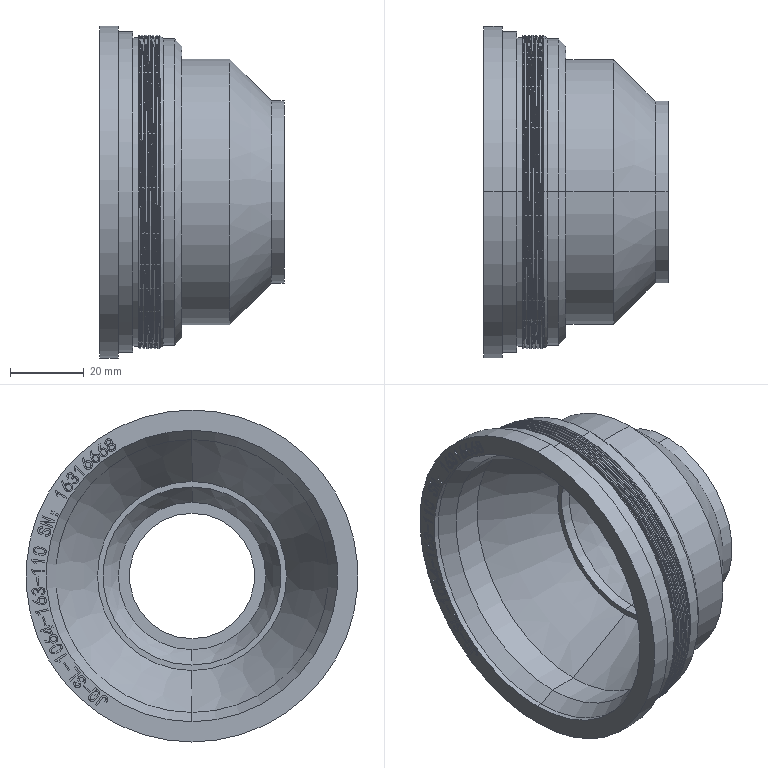Part | NX | features BREP 1 | 1 solid | 326 faces | box 50 x 90 x 90 mm | volume 73921 mm3 | plane 181 | spline 92 | cylinder 41 | cone 12 | commonest cylinder face diameters 85 x13 34 x2 40 x2 48.287 x2 49.5 x2 72 x2